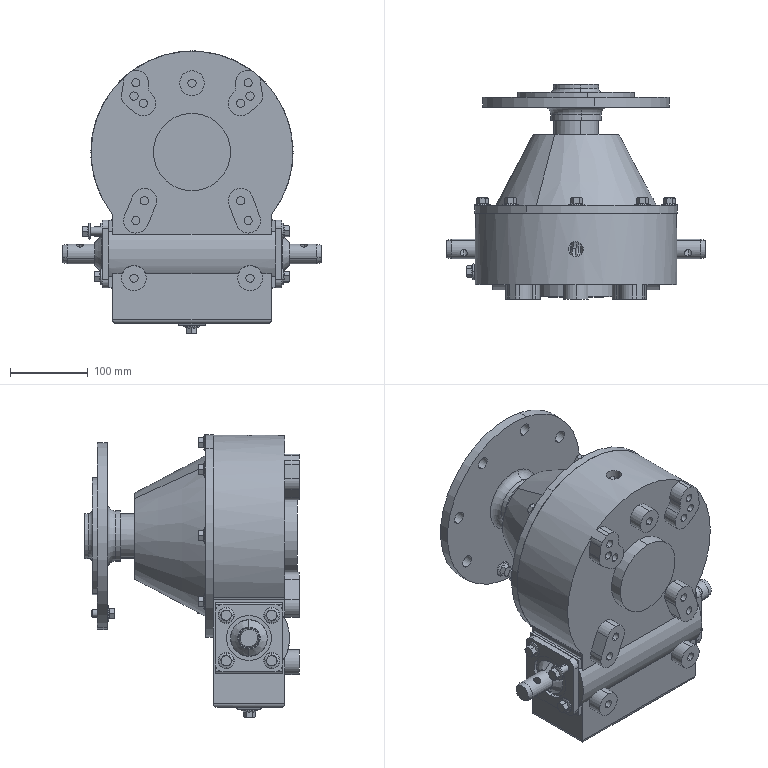Part | SolidWorks | features BaseBody 36 | 36 solids | 1469 faces | box 334 x 277.06 x 364.795 mm | volume 6574332 mm3 | cylinder 475 | plane 354 | spline 257 | cone 235 | torus 148 | commonest cylinder face diameters 223 x102 10 x56 8.5 x30 10.62 x22 32.08 x20 16 x18